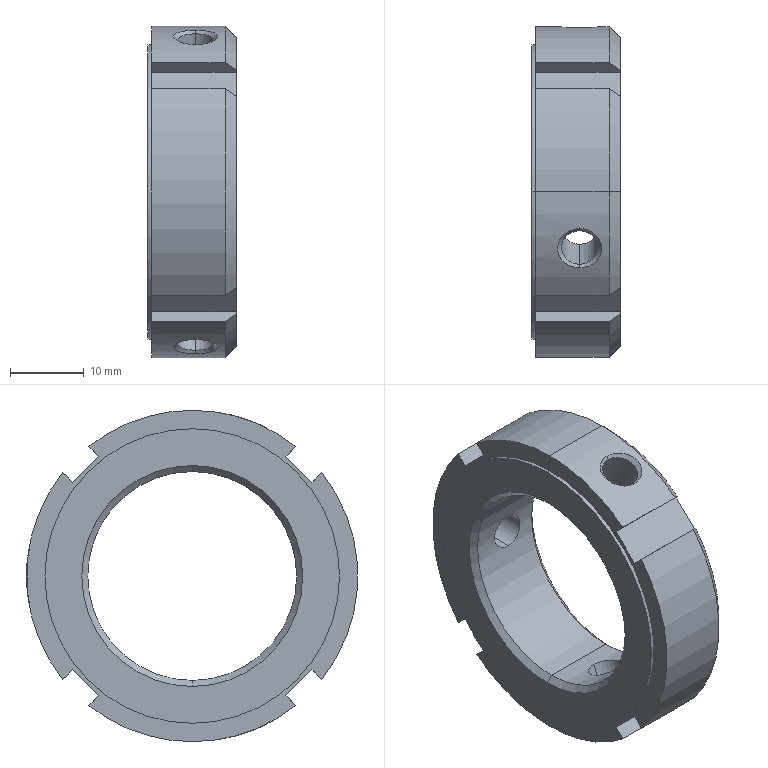Part | STEP file | _PLNY30x | 1 solid | 50 faces | box 12 x 45 x 45 mm | volume 10207 mm3 | plane 16 | cone 16 | cylinder 16 | torus 2 | commonest cylinder face diameters 4.917 x6 45 x6 28.376 x2 40 x2